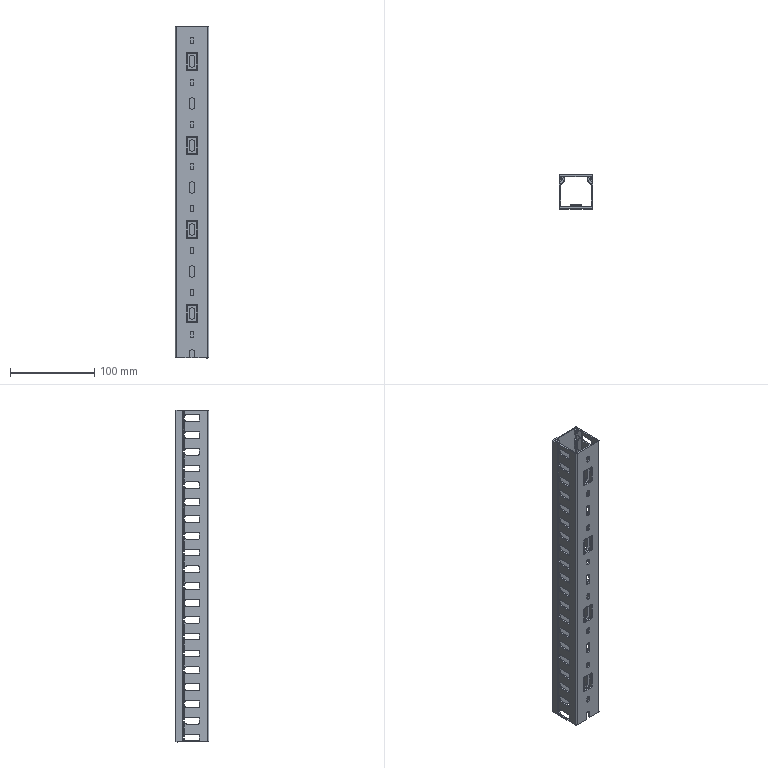Part | SolidWorks | features BaseBody 2 | 2 solids | 1550 faces | box 40 x 40.1 x 395 mm | volume 108160 mm3 | cylinder 851 | plane 603 | sphere 64 | torus 32 | commonest cylinder face diameters 4 x160 1 x132 3.6 x126 3 x124 1.464 x96 1.4 x84